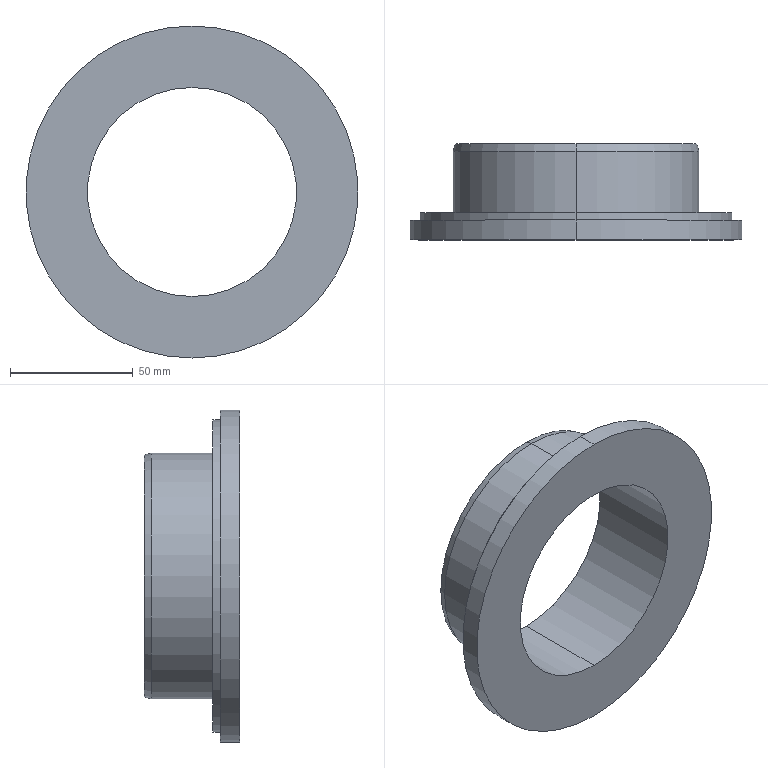Part | SolidWorks | features Chamfer 1, Revolution 1 | 1 solid | 14 faces | box 135 x 39 x 135 mm | volume 150743 mm3 | cylinder 8 | plane 4 | cone 2 | commonest cylinder face diameters 85 x2 100 x2 127 x2 135 x2
STEP:
#1=CARTESIAN_POINT('',(0.,31.,49.196));
#2=VERTEX_POINT('',#1);
#3=CARTESIAN_POINT('',(0.,31.,-49.196));
#4=VERTEX_POINT('',#3);
#5=CARTESIAN_POINT('',(0.,31.,0.));
#6=DIRECTION('',(0.,1.,0.));
#7=DIRECTION('',(0.,0.,1.));
#8=AXIS2_PLACEMENT_3D('',#5,#6,#7);
#9=CIRCLE('',#8,49.196);
#10=EDGE_CURVE('',#2,#4,#9,.T.);
#11=ORIENTED_EDGE('',*,*,#10,.F.);
#12=CARTESIAN_POINT('',(0.,28.,50.));
#13=VERTEX_POINT('',#12);
#14=CARTESIAN_POINT('',(0.,28.,50.));
#15=DIRECTION('',(0.,-0.9659,0.2588));
#16=VECTOR('',#15,1000.);
#17=LINE('',#14,#16);
#18=EDGE_CURVE('',#2,#13,#17,.T.);
#19=ORIENTED_EDGE('',*,*,#18,.T.);
#20=CARTESIAN_POINT('',(0.,28.,-50.));
#21=VERTEX_POINT('',#20);
#22=CARTESIAN_POINT('',(0.,28.,0.));
#23=DIRECTION('',(0.,-1.,0.));
#24=DIRECTION('',(0.,0.,1.));
#25=AXIS2_PLACEMENT_3D('',#22,#23,#24);
#26=CIRCLE('',#25,50.);
#27=EDGE_CURVE('',#21,#13,#26,.T.);
#28=ORIENTED_EDGE('',*,*,#27,.F.);
#29=CARTESIAN_POINT('',(0.,28.,-50.));
#30=DIRECTION('',(0.,-0.9659,-0.2588));
#31=VECTOR('',#30,1000.);
#32=LINE('',#29,#31);
#33=EDGE_CURVE('',#4,#21,#32,.T.);
#34=ORIENTED_EDGE('',*,*,#33,.F.);
#35=EDGE_LOOP('',(#11,#19,#28,#34));
#36=FACE_OUTER_BOUND('',#35,.T.);
#37=CARTESIAN_POINT('',(0.,28.,0.));
#38=DIRECTION('',(0.,-1.,0.));
#39=DIRECTION('',(0.,0.,-1.));
#40=AXIS2_PLACEMENT_3D('',#37,#38,#39);
#41=CONICAL_SURFACE('',#40,50.,0.2618);
#42=ADVANCED_FACE('',(#36),#41,.T.);
#43=CARTESIAN_POINT('',(0.,3.,-63.5));
#44=VERTEX_POINT('',#43);
#45=CARTESIAN_POINT('',(0.,3.,63.5));
#46=VERTEX_POINT('',#45);
#47=CARTESIAN_POINT('',(0.,3.,0.));
#48=DIRECTION('',(0.,-1.,0.));
#49=DIRECTION('',(0.,0.,-1.));
#50=AXIS2_PLACEMENT_3D('',#47,#48,#49);
#51=CIRCLE('',#50,63.5);
#52=EDGE_CURVE('',#44,#46,#51,.T.);
#53=ORIENTED_EDGE('',*,*,#52,.T.);
#54=CARTESIAN_POINT('',(0.,0.,63.5));
#55=VERTEX_POINT('',#54);
#56=CARTESIAN_POINT('',(0.,0.,63.5));
#57=DIRECTION('',(0.,-1.,0.));
#58=VECTOR('',#57,1000.);
#59=LINE('',#56,#58);
#60=EDGE_CURVE('',#46,#55,#59,.T.);
#61=ORIENTED_EDGE('',*,*,#60,.T.);
#62=CARTESIAN_POINT('',(0.,0.,-63.5));
#63=VERTEX_POINT('',#62);
#64=CARTESIAN_POINT('',(0.,0.,0.));
#65=DIRECTION('',(0.,-1.,0.));
#66=DIRECTION('',(0.,0.,-1.));
#67=AXIS2_PLACEMENT_3D('',#64,#65,#66);
#68=CIRCLE('',#67,63.5);
#69=EDGE_CURVE('',#63,#55,#68,.T.);
#70=ORIENTED_EDGE('',*,*,#69,.F.);
#71=CARTESIAN_POINT('',(0.,0.,-63.5));
#72=DIRECTION('',(0.,-1.,0.));
#73=VECTOR('',#72,1000.);
#74=LINE('',#71,#73);
#75=EDGE_CURVE('',#44,#63,#74,.T.);
#76=ORIENTED_EDGE('',*,*,#75,.F.);
#77=EDGE_LOOP('',(#53,#61,#70,#76));
#78=FACE_OUTER_BOUND('',#77,.T.);
#79=CARTESIAN_POINT('',(0.,0.,0.));
#80=DIRECTION('',(0.,-1.,0.));
#81=DIRECTION('',(0.,0.,-1.));
#82=AXIS2_PLACEMENT_3D('',#79,#80,#81);
#83=CYLINDRICAL_SURFACE('',#82,63.5);
#84=ADVANCED_FACE('',(#78),#83,.T.);
#85=CARTESIAN_POINT('',(0.,0.,-67.5));
#86=VERTEX_POINT('',#85);
#87=CARTESIAN_POINT('',(0.,0.,67.5));
#88=VERTEX_POINT('',#87);
#89=CARTESIAN_POINT('',(0.,0.,0.));
#90=DIRECTION('',(0.,-1.,0.));
#91=DIRECTION('',(0.,0.,-1.));
#92=AXIS2_PLACEMENT_3D('',#89,#90,#91);
#93=CIRCLE('',#92,67.5);
#94=EDGE_CURVE('',#86,#88,#93,.T.);
#95=ORIENTED_EDGE('',*,*,#94,.T.);
#96=CARTESIAN_POINT('',(0.,-8.,67.5));
#97=VERTEX_POINT('',#96);
#98=CARTESIAN_POINT('',(0.,0.,67.5));
#99=DIRECTION('',(0.,-1.,0.));
#100=VECTOR('',#99,1000.);
#101=LINE('',#98,#100);
#102=EDGE_CURVE('',#88,#97,#101,.T.);
#103=ORIENTED_EDGE('',*,*,#102,.T.);
#104=CARTESIAN_POINT('',(0.,-8.,-67.5));
#105=VERTEX_POINT('',#104);
#106=CARTESIAN_POINT('',(0.,-8.,0.));
#107=DIRECTION('',(0.,-1.,0.));
#108=DIRECTION('',(0.,0.,-1.));
#109=AXIS2_PLACEMENT_3D('',#106,#107,#108);
#110=CIRCLE('',#109,67.5);
#111=EDGE_CURVE('',#105,#97,#110,.T.);
#112=ORIENTED_EDGE('',*,*,#111,.F.);
#113=CARTESIAN_POINT('',(0.,0.,-67.5));
#114=DIRECTION('',(0.,-1.,0.));
#115=VECTOR('',#114,1000.);
#116=LINE('',#113,#115);
#117=EDGE_CURVE('',#86,#105,#116,.T.);
#118=ORIENTED_EDGE('',*,*,#117,.F.);
#119=EDGE_LOOP('',(#95,#103,#112,#118));
#120=FACE_OUTER_BOUND('',#119,.T.);
#121=CARTESIAN_POINT('',(0.,0.,0.));
#122=DIRECTION('',(0.,-1.,0.));
#123=DIRECTION('',(0.,0.,-1.));
#124=AXIS2_PLACEMENT_3D('',#121,#122,#123);
#125=CYLINDRICAL_SURFACE('',#124,67.5);
#126=ADVANCED_FACE('',(#120),#125,.T.);
#127=CARTESIAN_POINT('',(0.,31.,42.5));
#128=VERTEX_POINT('',#127);
#129=CARTESIAN_POINT('',(0.,31.,-42.5));
#130=VERTEX_POINT('',#129);
#131=CARTESIAN_POINT('',(0.,31.,0.));
#132=DIRECTION('',(0.,-1.,0.));
#133=DIRECTION('',(0.,0.,-1.));
#134=AXIS2_PLACEMENT_3D('',#131,#132,#133);
#135=CIRCLE('',#134,42.5);
#136=EDGE_CURVE('',#128,#130,#135,.T.);
#137=ORIENTED_EDGE('',*,*,#136,.F.);
#138=CARTESIAN_POINT('',(0.,-8.,42.5));
#139=VERTEX_POINT('',#138);
#140=CARTESIAN_POINT('',(0.,0.,42.5));
#141=DIRECTION('',(0.,-1.,0.));
#142=VECTOR('',#141,1000.);
#143=LINE('',#140,#142);
#144=EDGE_CURVE('',#128,#139,#143,.T.);
#145=ORIENTED_EDGE('',*,*,#144,.T.);
#146=CARTESIAN_POINT('',(0.,-8.,-42.5));
#147=VERTEX_POINT('',#146);
#148=CARTESIAN_POINT('',(0.,-8.,0.));
#149=DIRECTION('',(0.,-1.,0.));
#150=DIRECTION('',(0.,0.,-1.));
#151=AXIS2_PLACEMENT_3D('',#148,#149,#150);
#152=CIRCLE('',#151,42.5);
#153=EDGE_CURVE('',#139,#147,#152,.T.);
#154=ORIENTED_EDGE('',*,*,#153,.T.);
#155=CARTESIAN_POINT('',(0.,0.,-42.5));
#156=DIRECTION('',(0.,-1.,0.));
#157=VECTOR('',#156,1000.);
#158=LINE('',#155,#157);
#159=EDGE_CURVE('',#130,#147,#158,.T.);
#160=ORIENTED_EDGE('',*,*,#159,.F.);
#161=EDGE_LOOP('',(#137,#145,#154,#160));
#162=FACE_OUTER_BOUND('',#161,.T.);
#163=CARTESIAN_POINT('',(0.,0.,0.));
#164=DIRECTION('',(0.,-1.,0.));
#165=DIRECTION('',(0.,0.,-1.));
#166=AXIS2_PLACEMENT_3D('',#163,#164,#165);
#167=CYLINDRICAL_SURFACE('',#166,42.5);
#168=ADVANCED_FACE('',(#162),#167,.F.);
#169=ORIENTED_EDGE('',*,*,#27,.T.);
#170=CARTESIAN_POINT('',(0.,3.,50.));
#171=VERTEX_POINT('',#170);
#172=CARTESIAN_POINT('',(0.,0.,50.));
#173=DIRECTION('',(0.,-1.,0.));
#174=VECTOR('',#173,1000.);
#175=LINE('',#172,#174);
#176=EDGE_CURVE('',#13,#171,#175,.T.);
#177=ORIENTED_EDGE('',*,*,#176,.T.);
#178=CARTESIAN_POINT('',(0.,3.,-50.));
#179=VERTEX_POINT('',#178);
#180=CARTESIAN_POINT('',(0.,3.,0.));
#181=DIRECTION('',(0.,-1.,0.));
#182=DIRECTION('',(0.,0.,-1.));
#183=AXIS2_PLACEMENT_3D('',#180,#181,#182);
#184=CIRCLE('',#183,50.);
#185=EDGE_CURVE('',#179,#171,#184,.T.);
#186=ORIENTED_EDGE('',*,*,#185,.F.);
#187=CARTESIAN_POINT('',(0.,0.,-50.));
#188=DIRECTION('',(0.,-1.,0.));
#189=VECTOR('',#188,1000.);
#190=LINE('',#187,#189);
#191=EDGE_CURVE('',#21,#179,#190,.T.);
#192=ORIENTED_EDGE('',*,*,#191,.F.);
#193=EDGE_LOOP('',(#169,#177,#186,#192));
#194=FACE_OUTER_BOUND('',#193,.T.);
#195=CARTESIAN_POINT('',(0.,0.,0.));
#196=DIRECTION('',(0.,-1.,0.));
#197=DIRECTION('',(0.,0.,-1.));
#198=AXIS2_PLACEMENT_3D('',#195,#196,#197);
#199=CYLINDRICAL_SURFACE('',#198,50.);
#200=ADVANCED_FACE('',(#194),#199,.T.);
#201=ORIENTED_EDGE('',*,*,#176,.F.);
#202=CARTESIAN_POINT('',(0.,28.,0.));
#203=DIRECTION('',(0.,-1.,0.));
#204=DIRECTION('',(0.,0.,1.));
#205=AXIS2_PLACEMENT_3D('',#202,#203,#204);
#206=CIRCLE('',#205,50.);
#207=EDGE_CURVE('',#13,#21,#206,.T.);
#208=ORIENTED_EDGE('',*,*,#207,.T.);
#209=ORIENTED_EDGE('',*,*,#191,.T.);
#210=CARTESIAN_POINT('',(0.,3.,0.));
#211=DIRECTION('',(0.,-1.,0.));
#212=DIRECTION('',(0.,0.,-1.));
#213=AXIS2_PLACEMENT_3D('',#210,#211,#212);
#214=CIRCLE('',#213,50.);
#215=EDGE_CURVE('',#171,#179,#214,.T.);
#216=ORIENTED_EDGE('',*,*,#215,.F.);
#217=EDGE_LOOP('',(#201,#208,#209,#216));
#218=FACE_OUTER_BOUND('',#217,.T.);
#219=CARTESIAN_POINT('',(0.,0.,0.));
#220=DIRECTION('',(0.,-1.,0.));
#221=DIRECTION('',(0.,0.,-1.));
#222=AXIS2_PLACEMENT_3D('',#219,#220,#221);
#223=CYLINDRICAL_SURFACE('',#222,50.);
#224=ADVANCED_FACE('',(#218),#223,.T.);
#225=CARTESIAN_POINT('',(0.,31.,0.));
#226=DIRECTION('',(0.,1.,0.));
#227=DIRECTION('',(0.,0.,1.));
#228=AXIS2_PLACEMENT_3D('',#225,#226,#227);
#229=CIRCLE('',#228,49.196);
#230=EDGE_CURVE('',#4,#2,#229,.T.);
#231=ORIENTED_EDGE('',*,*,#230,.T.);
#232=ORIENTED_EDGE('',*,*,#10,.T.);
#233=EDGE_LOOP('',(#231,#232));
#234=FACE_OUTER_BOUND('',#233,.T.);
#235=CARTESIAN_POINT('',(0.,31.,0.));
#236=DIRECTION('',(0.,-1.,0.));
#237=DIRECTION('',(0.,0.,-1.));
#238=AXIS2_PLACEMENT_3D('',#235,#236,#237);
#239=CIRCLE('',#238,42.5);
#240=EDGE_CURVE('',#130,#128,#239,.T.);
#241=ORIENTED_EDGE('',*,*,#240,.T.);
#242=ORIENTED_EDGE('',*,*,#136,.T.);
#243=EDGE_LOOP('',(#241,#242));
#244=FACE_BOUND('',#243,.T.);
#245=CARTESIAN_POINT('',(42.5,31.,0.));
#246=DIRECTION('',(0.,1.,0.));
#247=DIRECTION('',(0.,0.,1.));
#248=AXIS2_PLACEMENT_3D('',#245,#246,#247);
#249=PLANE('',#248);
#250=ADVANCED_FACE('',(#234,#244),#249,.T.);
#251=ORIENTED_EDGE('',*,*,#144,.F.);
#252=ORIENTED_EDGE('',*,*,#240,.F.);
#253=ORIENTED_EDGE('',*,*,#159,.T.);
#254=CARTESIAN_POINT('',(0.,-8.,0.));
#255=DIRECTION('',(0.,-1.,0.));
#256=DIRECTION('',(0.,0.,-1.));
#257=AXIS2_PLACEMENT_3D('',#254,#255,#256);
#258=CIRCLE('',#257,42.5);
#259=EDGE_CURVE('',#147,#139,#258,.T.);
#260=ORIENTED_EDGE('',*,*,#259,.T.);
#261=EDGE_LOOP('',(#251,#252,#253,#260));
#262=FACE_OUTER_BOUND('',#261,.T.);
#263=CARTESIAN_POINT('',(0.,0.,0.));
#264=DIRECTION('',(0.,-1.,0.));
#265=DIRECTION('',(0.,0.,-1.));
#266=AXIS2_PLACEMENT_3D('',#263,#264,#265);
#267=CYLINDRICAL_SURFACE('',#266,42.5);
#268=ADVANCED_FACE('',(#262),#267,.F.);
#269=ORIENTED_EDGE('',*,*,#111,.T.);
#270=CARTESIAN_POINT('',(0.,-8.,0.));
#271=DIRECTION('',(0.,-1.,0.));
#272=DIRECTION('',(0.,0.,-1.));
#273=AXIS2_PLACEMENT_3D('',#270,#271,#272);
#274=CIRCLE('',#273,67.5);
#275=EDGE_CURVE('',#97,#105,#274,.T.);
#276=ORIENTED_EDGE('',*,*,#275,.T.);
#277=EDGE_LOOP('',(#269,#276));
#278=FACE_OUTER_BOUND('',#277,.T.);
#279=ORIENTED_EDGE('',*,*,#259,.F.);
#280=ORIENTED_EDGE('',*,*,#153,.F.);
#281=EDGE_LOOP('',(#279,#280));
#282=FACE_BOUND('',#281,.T.);
#283=CARTESIAN_POINT('',(67.5,-8.,0.));
#284=DIRECTION('',(0.,-1.,0.));
#285=DIRECTION('',(0.,0.,-1.));
#286=AXIS2_PLACEMENT_3D('',#283,#284,#285);
#287=PLANE('',#286);
#288=ADVANCED_FACE('',(#278,#282),#287,.T.);
#289=ORIENTED_EDGE('',*,*,#102,.F.);
#290=CARTESIAN_POINT('',(0.,0.,0.));
#291=DIRECTION('',(0.,-1.,0.));
#292=DIRECTION('',(0.,0.,-1.));
#293=AXIS2_PLACEMENT_3D('',#290,#291,#292);
#294=CIRCLE('',#293,67.5);
#295=EDGE_CURVE('',#88,#86,#294,.T.);
#296=ORIENTED_EDGE('',*,*,#295,.T.);
#297=ORIENTED_EDGE('',*,*,#117,.T.);
#298=ORIENTED_EDGE('',*,*,#275,.F.);
#299=EDGE_LOOP('',(#289,#296,#297,#298));
#300=FACE_OUTER_BOUND('',#299,.T.);
#301=CARTESIAN_POINT('',(0.,0.,0.));
#302=DIRECTION('',(0.,-1.,0.));
#303=DIRECTION('',(0.,0.,-1.));
#304=AXIS2_PLACEMENT_3D('',#301,#302,#303);
#305=CYLINDRICAL_SURFACE('',#304,67.5);
#306=ADVANCED_FACE('',(#300),#305,.T.);
#307=ORIENTED_EDGE('',*,*,#69,.T.);
#308=CARTESIAN_POINT('',(0.,0.,0.));
#309=DIRECTION('',(0.,-1.,0.));
#310=DIRECTION('',(0.,0.,-1.));
#311=AXIS2_PLACEMENT_3D('',#308,#309,#310);
#312=CIRCLE('',#311,63.5);
#313=EDGE_CURVE('',#55,#63,#312,.T.);
#314=ORIENTED_EDGE('',*,*,#313,.T.);
#315=EDGE_LOOP('',(#307,#314));
#316=FACE_BOUND('',#315,.T.);
#317=ORIENTED_EDGE('',*,*,#94,.F.);
#318=ORIENTED_EDGE('',*,*,#295,.F.);
#319=EDGE_LOOP('',(#317,#318));
#320=FACE_OUTER_BOUND('',#319,.T.);
#321=CARTESIAN_POINT('',(63.5,0.,0.));
#322=DIRECTION('',(0.,1.,0.));
#323=DIRECTION('',(0.,0.,1.));
#324=AXIS2_PLACEMENT_3D('',#321,#322,#323);
#325=PLANE('',#324);
#326=ADVANCED_FACE('',(#316,#320),#325,.T.);
#327=ORIENTED_EDGE('',*,*,#60,.F.);
#328=CARTESIAN_POINT('',(0.,3.,0.));
#329=DIRECTION('',(0.,-1.,0.));
#330=DIRECTION('',(0.,0.,-1.));
#331=AXIS2_PLACEMENT_3D('',#328,#329,#330);
#332=CIRCLE('',#331,63.5);
#333=EDGE_CURVE('',#46,#44,#332,.T.);
#334=ORIENTED_EDGE('',*,*,#333,.T.);
#335=ORIENTED_EDGE('',*,*,#75,.T.);
#336=ORIENTED_EDGE('',*,*,#313,.F.);
#337=EDGE_LOOP('',(#327,#334,#335,#336));
#338=FACE_OUTER_BOUND('',#337,.T.);
#339=CARTESIAN_POINT('',(0.,0.,0.));
#340=DIRECTION('',(0.,-1.,0.));
#341=DIRECTION('',(0.,0.,-1.));
#342=AXIS2_PLACEMENT_3D('',#339,#340,#341);
#343=CYLINDRICAL_SURFACE('',#342,63.5);
#344=ADVANCED_FACE('',(#338),#343,.T.);
#345=ORIENTED_EDGE('',*,*,#185,.T.);
#346=ORIENTED_EDGE('',*,*,#215,.T.);
#347=EDGE_LOOP('',(#345,#346));
#348=FACE_BOUND('',#347,.T.);
#349=ORIENTED_EDGE('',*,*,#52,.F.);
#350=ORIENTED_EDGE('',*,*,#333,.F.);
#351=EDGE_LOOP('',(#349,#350));
#352=FACE_OUTER_BOUND('',#351,.T.);
#353=CARTESIAN_POINT('',(50.,3.,0.));
#354=DIRECTION('',(0.,1.,0.));
#355=DIRECTION('',(0.,0.,1.));
#356=AXIS2_PLACEMENT_3D('',#353,#354,#355);
#357=PLANE('',#356);
#358=ADVANCED_FACE('',(#348,#352),#357,.T.);
#359=ORIENTED_EDGE('',*,*,#18,.F.);
#360=ORIENTED_EDGE('',*,*,#230,.F.);
#361=ORIENTED_EDGE('',*,*,#33,.T.);
#362=ORIENTED_EDGE('',*,*,#207,.F.);
#363=EDGE_LOOP('',(#359,#360,#361,#362));
#364=FACE_OUTER_BOUND('',#363,.T.);
#365=CARTESIAN_POINT('',(0.,28.,0.));
#366=DIRECTION('',(0.,-1.,0.));
#367=DIRECTION('',(0.,0.,-1.));
#368=AXIS2_PLACEMENT_3D('',#365,#366,#367);
#369=CONICAL_SURFACE('',#368,50.,0.2618);
#370=ADVANCED_FACE('',(#364),#369,.T.);
#371=CLOSED_SHELL('',(#42,#84,#126,#168,#200,#224,#250,#268,#288,#306,#326,#344,#358,#370));
#372=MANIFOLD_SOLID_BREP('',#371);
#373=CARTESIAN_POINT('',(0.,0.,0.));
#374=DIRECTION('',(0.,0.,1.));
#375=DIRECTION('',(1.,0.,0.));
#376=AXIS2_PLACEMENT_3D('',#373,#374,#375);
#377=(LENGTH_UNIT()NAMED_UNIT(*)SI_UNIT(.MILLI.,.METRE.));
#378=UNCERTAINTY_MEASURE_WITH_UNIT(LENGTH_MEASURE(0.00001),#377,'','');
#379=(NAMED_UNIT(*)PLANE_ANGLE_UNIT()SI_UNIT($,.RADIAN.));
#380=(NAMED_UNIT(*)SI_UNIT($,.STERADIAN.)SOLID_ANGLE_UNIT());
#381=(GEOMETRIC_REPRESENTATION_CONTEXT(3)GLOBAL_UNCERTAINTY_ASSIGNED_CONTEXT((#378))GLOBAL_UNIT_ASSIGNED_CONTEXT((#377,#379,#380))REPRESENTATION_CONTEXT('',''));
#382=ADVANCED_BREP_SHAPE_REPRESENTATION('',(#372,#376),#381);